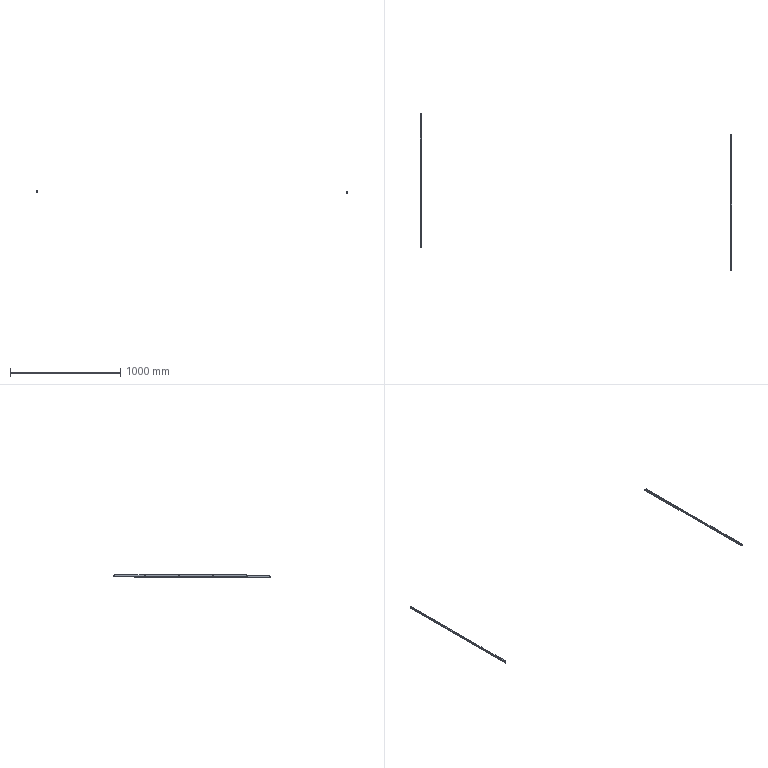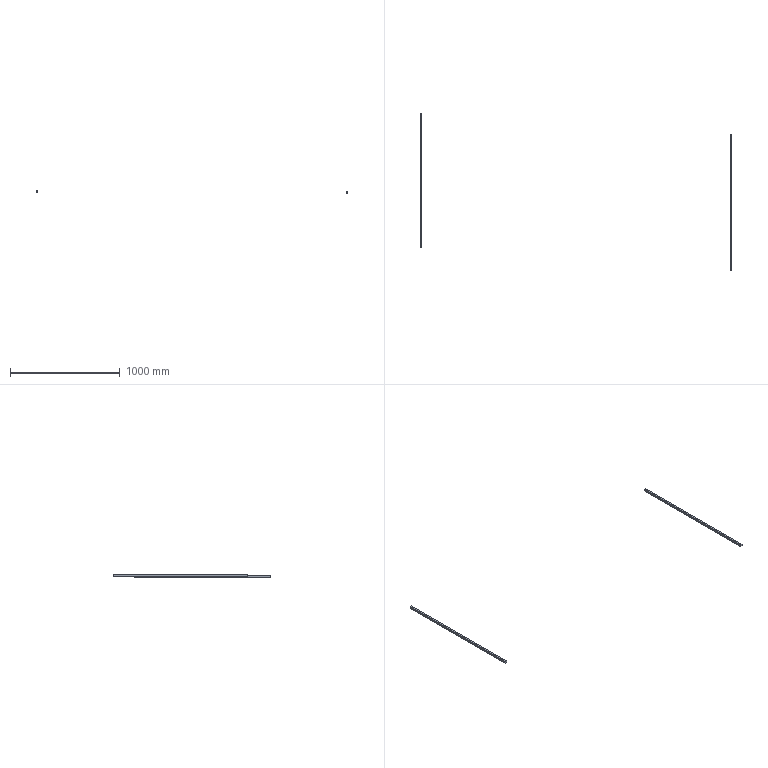CAM job | NX | 3+2 milling, drilling | part box 2829 x 1430 x 20 mm | stock box 2835 x 1435 x 24 mm
Tools:
number,name,description,diameter,corner_radius,flute_length,length,flutes
2,D8-25-D8-60-3T-ROUGH,D8-25-D8-60-3T-粗,8.0,0.0,25.0,60.0,2
3,D8-25-D8-60-3T-FINISH,D8-25-D8-60-3T,8.0,0.0,25.0,60.0,3
1,D16-48-D16-100-3T-FINISH,D16-48-D16-100-3T,16.0,0.0,48.0,100.0,3
0,钻头D3.3-45-73,钻刀D3.3-45-73,3.3,0.0,45.0,73.0,2
5,钻头D4.3-54-83,钻刀D4.3-54-83,4.3,0.0,54.0,83.0,2
6,上排M4-13-D5-52,上排M4-13-D5-52,4.0,0.0,14.0,17.0,2
4,倒角D6-90度,倒角D6-90度,6.0,0.0,5.0,50.0,2
Operations:
program,operation,operation_type,tool,method,geometry_group,spindle_rpm,surface_speed,feed_per_tooth,feed_cut,feed_plunge,cut_length_mm,path_length_mm,cut_time_min,machine_time_min
A1,PLANAR_MILL,PlanarMilling,D16-48-D16-100-3T-FINISH,METHOD,A-G54,4000.0,201.0,0.0833,1000.0,100.0,1057.0,1093.0,1.057,1.061
A1,动态粗,CavityMilling,D8-25-D8-60-3T-ROUGH,METHOD,WORKPIECE,6500.0,100.0,0.1178,3000.0,100.0,6276.398,6349.398,2.092,2.099
A1,PLANAR_MILL_1,PlanarMilling,D8-25-D8-60-3T-FINISH,METHOD,WORKPIECE,4500.0,113.0,0.0741,1000.0,100.0,2105.856,2175.856,2.106,2.113
A1,PLANAR_MILL_1_COPY,PlanarMilling,倒角D6-90度,METHOD,WORKPIECE,4500.0,113.0,0.0741,1000.0,100.0,2085.485,2124.485,2.086,2.089
B1,PLANAR_MILL_COPY,PlanarMilling,D16-48-D16-100-3T-FINISH,METHOD,B-G55,4000.0,201.0,0.0833,1000.0,100.0,3171.0,5378.8,3.171,3.392
B1,PLANAR_MILL_COPY_COPY,PlanarMilling,D16-48-D16-100-3T-FINISH,METHOD,B-G55,4000.0,201.0,0.0833,1000.0,100.0,1057.0,1093.0,1.057,1.061
B1,PLANAR_MILL_2,PlanarMilling,D8-25-D8-60-3T-FINISH,METHOD,B-G55,4500.0,113.0,0.0889,1200.0,100.0,1814.4,2539.994,1.512,1.585
B1,PLANAR_MILL_2_COPY,PlanarMilling,D8-25-D8-60-3T-FINISH,METHOD,B-G55,4500.0,113.0,0.0889,800.0,100.0,120.12,784.735,0.1501,0.2166
B1,DRILLING,Operation,倒角D6-90度,METHOD,B-G55,2000.0,37.0,0.05,200.0,0.0,25.0,1099.572,0.125,0.2325
B1,PLANAR_MILL_3,PlanarMilling,倒角D6-90度,METHOD,B-G55,3000.0,56.0,0.1667,1000.0,100.0,2142.832,3082.832,2.143,2.237
B1,DRILLING_COPY,Operation,钻头D4.3-54-83,METHOD,B-G55,2000.0,37.0,0.05,200.0,0.0,90.0,1229.572,0.45,0.564
B1,DRILLING_COPY_COPY,Operation,上排M4-13-D5-52,METHOD,B-G55,300.0,3.0,0.0012,0.7,0.0,65.0,1179.572,92.857,92.969
C1,PLANAR_MILL_COPY_1,PlanarMilling,D16-48-D16-100-3T-FINISH,METHOD,WORKPIECE_56,4000.0,201.0,0.0833,1000.0,100.0,1251.0,1307.0,1.251,1.257
C1,动态粗_COPY,CavityMilling,D8-25-D8-60-3T-ROUGH,METHOD,WORKPIECE_56,6500.0,100.0,0.1178,3000.0,100.0,7498.41,7591.81,2.499,2.509
C1,PLANAR_MILL_1_COPY_1,PlanarMilling,D8-25-D8-60-3T-FINISH,METHOD,WORKPIECE_56,4500.0,113.0,0.0741,1000.0,100.0,2503.856,2593.856,2.504,2.513
C1,PLANAR_MILL_1_COPY_COPY,PlanarMilling,倒角D6-90度,METHOD,WORKPIECE_56,4500.0,113.0,0.0741,1000.0,100.0,2483.485,2542.485,2.483,2.489
D1,PLANAR_MILL_COPY_COPY_1,PlanarMilling,D16-48-D16-100-3T-FINISH,METHOD,WORKPIECE_57,4000.0,201.0,0.0833,1000.0,100.0,5004.0,8988.8,5.004,5.402
D1,PLANAR_MILL_COPY_COPY_1_COPY,PlanarMilling,D16-48-D16-100-3T-FINISH,METHOD,WORKPIECE_57,4000.0,201.0,0.0833,1000.0,100.0,1251.0,1315.0,1.251,1.257
D1,PLANAR_MILL_2_COPY_1,PlanarMilling,D8-25-D8-60-3T-FINISH,METHOD,WORKPIECE_57,4500.0,113.0,0.0889,1200.0,100.0,1512.0,3112.136,1.26,1.42
D1,PLANAR_MILL_2_COPY_1_COPY,PlanarMilling,D8-25-D8-60-3T-FINISH,METHOD,WORKPIECE_57,4500.0,113.0,0.0741,1000.0,100.0,200.0,1764.389,0.2,0.3564
D1,PLANAR_MILL_3_COPY,PlanarMilling,倒角D6-90度,METHOD,WORKPIECE_57,3000.0,56.0,0.1667,1000.0,100.0,2500.832,3644.82,2.501,2.615
E1,PLANAR_MILL_COPY_2,PlanarMilling,D16-48-D16-100-3T-FINISH,METHOD,E-G58,4000.0,201.0,0.0833,1000.0,100.0,1271.0,1327.0,1.271,1.277
E1,动态粗_COPY_1,CavityMilling,D8-25-D8-60-3T-ROUGH,METHOD,WORKPIECE_58,6500.0,100.0,0.1178,3000.0,100.0,7559.547,7652.948,2.52,2.529
E1,PLANAR_MILL_1_COPY_2,PlanarMilling,D8-25-D8-60-3T-FINISH,METHOD,WORKPIECE_58,4500.0,113.0,0.0741,1000.0,100.0,5067.713,5251.854,5.068,5.086
E1,PLANAR_MILL_1_COPY_COPY_1,PlanarMilling,倒角D6-90度,METHOD,WORKPIECE_58,4500.0,113.0,0.0741,1000.0,100.0,2513.485,2572.485,2.514,2.519
G1,PLANAR_MILL_COPY_COPY_1_COPY_1,PlanarMilling,D16-48-D16-100-3T-FINISH,METHOD,WORKPIECE_59,4000.0,201.0,0.0833,1000.0,100.0,5064.0,9253.8,5.064,5.483
G1,PLANAR_MILL_COPY_COPY_1_COPY_1_COPY,PlanarMilling,D16-48-D16-100-3T-FINISH,METHOD,WORKPIECE_59,4000.0,201.0,0.0833,1000.0,100.0,1266.0,1370.0,1.266,1.276
G1,PLANAR_MILL_2_COPY_1_COPY_1,PlanarMilling,D8-25-D8-60-3T-FINISH,METHOD,WORKPIECE_59,4500.0,113.0,0.0889,1200.0,100.0,1512.0,3327.136,1.26,1.442
G1,PLANAR_MILL_2_COPY_1_COPY_1_COPY,PlanarMilling,D8-25-D8-60-3T-FINISH,METHOD,WORKPIECE_59,4500.0,113.0,0.0593,800.0,100.0,192.0,1970.278,0.24,0.4178
G1,PLANAR_MILL_3_COPY_COPY,PlanarMilling,倒角D6-90度,METHOD,WORKPIECE_59,3000.0,56.0,0.1667,1000.0,100.0,2530.832,3861.832,2.531,2.664
工装1,DRILLING_1,Operation,倒角D6-90度,METHOD,GZ1,2000.0,37.0,0.05,200.0,0.0,35.0,1048.18,0.175,0.2763
工装1,DRILLING_1_COPY,Operation,钻头D3.3-45-73,METHOD,GZ1,2000.0,37.0,0.05,200.0,0.0,112.0,1202.18,0.56,0.669
工装1,DRILLING_1_COPY_COPY,Operation,上排M4-13-D5-52,METHOD,GZ1,300.0,3.0,0.35,210.0,0.0,56.0,1090.18,0.2667,0.3701